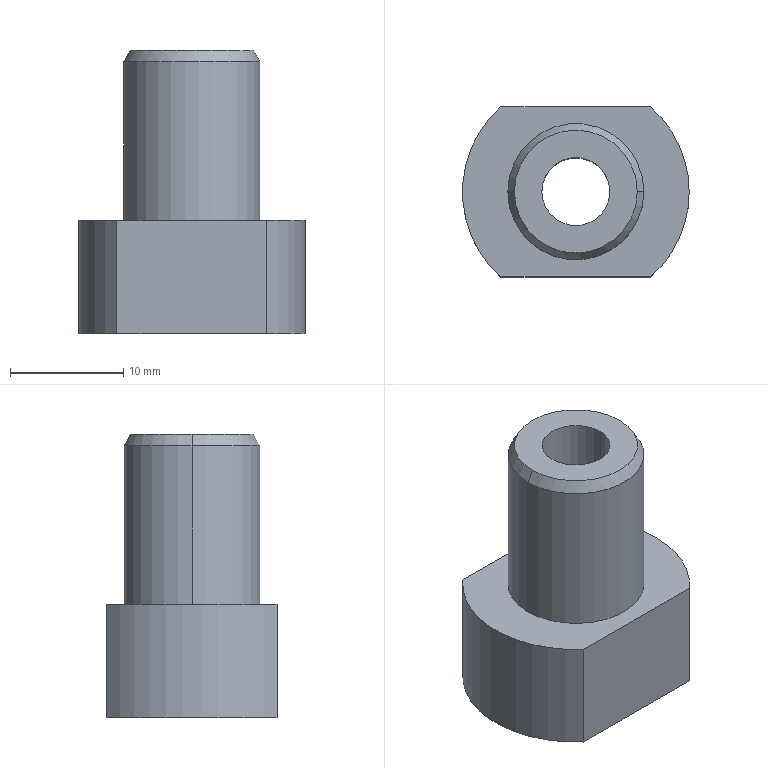Part | SolidWorks | features ICE 2, Chamfer 1, Extrusion 1 | 1 solid | 14 faces | box 20 x 15 x 25 mm | volume 3667 mm3 | cylinder 7 | plane 5 | cone 2 | commonest cylinder face diameters 20 x3 6 x2 12 x2
STEP:
#1=CARTESIAN_POINT('',(10.,0.,-10.));
#2=VERTEX_POINT('',#1);
#3=CARTESIAN_POINT('',(6.614,-7.5,-10.));
#4=VERTEX_POINT('',#3);
#5=CARTESIAN_POINT('',(0.,0.,-10.));
#6=DIRECTION('',(0.,0.,-1.));
#7=DIRECTION('',(-1.,0.,0.));
#8=AXIS2_PLACEMENT_3D('',#5,#6,#7);
#9=CIRCLE('',#8,10.);
#10=EDGE_CURVE('',#2,#4,#9,.T.);
#11=ORIENTED_EDGE('',*,*,#10,.F.);
#12=CARTESIAN_POINT('',(10.,0.,0.));
#13=VERTEX_POINT('',#12);
#14=CARTESIAN_POINT('',(10.,0.,-10.));
#15=DIRECTION('',(0.,0.,1.));
#16=VECTOR('',#15,1000.);
#17=LINE('',#14,#16);
#18=EDGE_CURVE('',#2,#13,#17,.T.);
#19=ORIENTED_EDGE('',*,*,#18,.T.);
#20=CARTESIAN_POINT('',(6.614,-7.5,0.));
#21=VERTEX_POINT('',#20);
#22=CARTESIAN_POINT('',(0.,0.,0.));
#23=DIRECTION('',(0.,0.,-1.));
#24=DIRECTION('',(-1.,0.,0.));
#25=AXIS2_PLACEMENT_3D('',#22,#23,#24);
#26=CIRCLE('',#25,10.);
#27=EDGE_CURVE('',#13,#21,#26,.T.);
#28=ORIENTED_EDGE('',*,*,#27,.T.);
#29=CARTESIAN_POINT('',(6.614,-7.5,-10.));
#30=DIRECTION('',(0.,0.,-1.));
#31=VECTOR('',#30,1000.);
#32=LINE('',#29,#31);
#33=EDGE_CURVE('',#21,#4,#32,.T.);
#34=ORIENTED_EDGE('',*,*,#33,.T.);
#35=EDGE_LOOP('',(#11,#19,#28,#34));
#36=FACE_OUTER_BOUND('',#35,.T.);
#37=CARTESIAN_POINT('',(0.,0.,-10.));
#38=DIRECTION('',(0.,0.,1.));
#39=DIRECTION('',(1.,0.,0.));
#40=AXIS2_PLACEMENT_3D('',#37,#38,#39);
#41=CYLINDRICAL_SURFACE('',#40,10.);
#42=ADVANCED_FACE('',(#36),#41,.T.);
#43=CARTESIAN_POINT('',(5.423,0.,15.));
#44=VERTEX_POINT('',#43);
#45=CARTESIAN_POINT('',(-5.423,0.,15.));
#46=VERTEX_POINT('',#45);
#47=CARTESIAN_POINT('',(0.,0.,15.));
#48=DIRECTION('',(0.,0.,1.));
#49=DIRECTION('',(1.,0.,0.));
#50=AXIS2_PLACEMENT_3D('',#47,#48,#49);
#51=CIRCLE('',#50,5.423);
#52=EDGE_CURVE('',#44,#46,#51,.T.);
#53=ORIENTED_EDGE('',*,*,#52,.F.);
#54=CARTESIAN_POINT('',(6.,0.,14.));
#55=VERTEX_POINT('',#54);
#56=CARTESIAN_POINT('',(5.423,0.,15.));
#57=DIRECTION('',(0.5,0.,-0.866));
#58=VECTOR('',#57,1000.);
#59=LINE('',#56,#58);
#60=EDGE_CURVE('',#44,#55,#59,.T.);
#61=ORIENTED_EDGE('',*,*,#60,.T.);
#62=CARTESIAN_POINT('',(-6.,0.,14.));
#63=VERTEX_POINT('',#62);
#64=CARTESIAN_POINT('',(0.,0.,14.));
#65=DIRECTION('',(0.,0.,-1.));
#66=DIRECTION('',(1.,0.,0.));
#67=AXIS2_PLACEMENT_3D('',#64,#65,#66);
#68=CIRCLE('',#67,6.);
#69=EDGE_CURVE('',#63,#55,#68,.T.);
#70=ORIENTED_EDGE('',*,*,#69,.F.);
#71=CARTESIAN_POINT('',(-5.423,0.,15.));
#72=DIRECTION('',(-0.5,0.,-0.866));
#73=VECTOR('',#72,1000.);
#74=LINE('',#71,#73);
#75=EDGE_CURVE('',#46,#63,#74,.T.);
#76=ORIENTED_EDGE('',*,*,#75,.F.);
#77=EDGE_LOOP('',(#53,#61,#70,#76));
#78=FACE_OUTER_BOUND('',#77,.T.);
#79=CARTESIAN_POINT('',(0.,0.,15.));
#80=DIRECTION('',(0.,0.,-1.));
#81=DIRECTION('',(-1.,0.,0.));
#82=AXIS2_PLACEMENT_3D('',#79,#80,#81);
#83=CONICAL_SURFACE('',#82,5.423,0.5236);
#84=ADVANCED_FACE('',(#78),#83,.T.);
#85=CARTESIAN_POINT('',(-3.,0.,15.));
#86=VERTEX_POINT('',#85);
#87=CARTESIAN_POINT('',(3.,0.,15.));
#88=VERTEX_POINT('',#87);
#89=CARTESIAN_POINT('',(0.,0.,15.));
#90=DIRECTION('',(0.,0.,1.));
#91=DIRECTION('',(1.,0.,0.));
#92=AXIS2_PLACEMENT_3D('',#89,#90,#91);
#93=CIRCLE('',#92,3.);
#94=EDGE_CURVE('',#86,#88,#93,.T.);
#95=ORIENTED_EDGE('',*,*,#94,.T.);
#96=CARTESIAN_POINT('',(3.,0.,-10.));
#97=VERTEX_POINT('',#96);
#98=CARTESIAN_POINT('',(3.,0.,15.));
#99=DIRECTION('',(0.,0.,-1.));
#100=VECTOR('',#99,1000.);
#101=LINE('',#98,#100);
#102=EDGE_CURVE('',#88,#97,#101,.T.);
#103=ORIENTED_EDGE('',*,*,#102,.T.);
#104=CARTESIAN_POINT('',(-3.,0.,-10.));
#105=VERTEX_POINT('',#104);
#106=CARTESIAN_POINT('',(0.,0.,-10.));
#107=DIRECTION('',(0.,0.,-1.));
#108=DIRECTION('',(-1.,0.,0.));
#109=AXIS2_PLACEMENT_3D('',#106,#107,#108);
#110=CIRCLE('',#109,3.);
#111=EDGE_CURVE('',#97,#105,#110,.T.);
#112=ORIENTED_EDGE('',*,*,#111,.T.);
#113=CARTESIAN_POINT('',(-3.,0.,15.));
#114=DIRECTION('',(0.,0.,-1.));
#115=VECTOR('',#114,1000.);
#116=LINE('',#113,#115);
#117=EDGE_CURVE('',#86,#105,#116,.T.);
#118=ORIENTED_EDGE('',*,*,#117,.F.);
#119=EDGE_LOOP('',(#95,#103,#112,#118));
#120=FACE_OUTER_BOUND('',#119,.T.);
#121=CARTESIAN_POINT('',(0.,0.,15.));
#122=DIRECTION('',(0.,0.,-1.));
#123=DIRECTION('',(-1.,0.,0.));
#124=AXIS2_PLACEMENT_3D('',#121,#122,#123);
#125=CYLINDRICAL_SURFACE('',#124,3.);
#126=ADVANCED_FACE('',(#120),#125,.F.);
#127=ORIENTED_EDGE('',*,*,#69,.T.);
#128=CARTESIAN_POINT('',(6.,0.,0.));
#129=VERTEX_POINT('',#128);
#130=CARTESIAN_POINT('',(6.,0.,15.));
#131=DIRECTION('',(0.,0.,-1.));
#132=VECTOR('',#131,1000.);
#133=LINE('',#130,#132);
#134=EDGE_CURVE('',#55,#129,#133,.T.);
#135=ORIENTED_EDGE('',*,*,#134,.T.);
#136=CARTESIAN_POINT('',(-6.,0.,0.));
#137=VERTEX_POINT('',#136);
#138=CARTESIAN_POINT('',(0.,0.,0.));
#139=DIRECTION('',(0.,0.,1.));
#140=DIRECTION('',(1.,0.,0.));
#141=AXIS2_PLACEMENT_3D('',#138,#139,#140);
#142=CIRCLE('',#141,6.);
#143=EDGE_CURVE('',#129,#137,#142,.T.);
#144=ORIENTED_EDGE('',*,*,#143,.T.);
#145=CARTESIAN_POINT('',(-6.,0.,15.));
#146=DIRECTION('',(0.,0.,-1.));
#147=VECTOR('',#146,1000.);
#148=LINE('',#145,#147);
#149=EDGE_CURVE('',#63,#137,#148,.T.);
#150=ORIENTED_EDGE('',*,*,#149,.F.);
#151=EDGE_LOOP('',(#127,#135,#144,#150));
#152=FACE_OUTER_BOUND('',#151,.T.);
#153=CARTESIAN_POINT('',(0.,0.,15.));
#154=DIRECTION('',(0.,0.,-1.));
#155=DIRECTION('',(-1.,0.,0.));
#156=AXIS2_PLACEMENT_3D('',#153,#154,#155);
#157=CYLINDRICAL_SURFACE('',#156,6.);
#158=ADVANCED_FACE('',(#152),#157,.T.);
#159=CARTESIAN_POINT('',(-6.614,-7.5,-10.));
#160=VERTEX_POINT('',#159);
#161=CARTESIAN_POINT('',(-6.614,7.5,-10.));
#162=VERTEX_POINT('',#161);
#163=CARTESIAN_POINT('',(0.,0.,-10.));
#164=DIRECTION('',(0.,0.,-1.));
#165=DIRECTION('',(-1.,0.,0.));
#166=AXIS2_PLACEMENT_3D('',#163,#164,#165);
#167=CIRCLE('',#166,10.);
#168=EDGE_CURVE('',#160,#162,#167,.T.);
#169=ORIENTED_EDGE('',*,*,#168,.F.);
#170=CARTESIAN_POINT('',(-6.614,-7.5,0.));
#171=VERTEX_POINT('',#170);
#172=CARTESIAN_POINT('',(-6.614,-7.5,-10.));
#173=DIRECTION('',(0.,0.,1.));
#174=VECTOR('',#173,1000.);
#175=LINE('',#172,#174);
#176=EDGE_CURVE('',#160,#171,#175,.T.);
#177=ORIENTED_EDGE('',*,*,#176,.T.);
#178=CARTESIAN_POINT('',(-6.614,7.5,0.));
#179=VERTEX_POINT('',#178);
#180=CARTESIAN_POINT('',(0.,0.,0.));
#181=DIRECTION('',(0.,0.,-1.));
#182=DIRECTION('',(-1.,0.,0.));
#183=AXIS2_PLACEMENT_3D('',#180,#181,#182);
#184=CIRCLE('',#183,10.);
#185=EDGE_CURVE('',#171,#179,#184,.T.);
#186=ORIENTED_EDGE('',*,*,#185,.T.);
#187=CARTESIAN_POINT('',(-6.614,7.5,-10.));
#188=DIRECTION('',(0.,0.,-1.));
#189=VECTOR('',#188,1000.);
#190=LINE('',#187,#189);
#191=EDGE_CURVE('',#179,#162,#190,.T.);
#192=ORIENTED_EDGE('',*,*,#191,.T.);
#193=EDGE_LOOP('',(#169,#177,#186,#192));
#194=FACE_OUTER_BOUND('',#193,.T.);
#195=CARTESIAN_POINT('',(0.,0.,-10.));
#196=DIRECTION('',(0.,0.,1.));
#197=DIRECTION('',(1.,0.,0.));
#198=AXIS2_PLACEMENT_3D('',#195,#196,#197);
#199=CYLINDRICAL_SURFACE('',#198,10.);
#200=ADVANCED_FACE('',(#194),#199,.T.);
#201=CARTESIAN_POINT('',(0.,0.,15.));
#202=DIRECTION('',(0.,0.,1.));
#203=DIRECTION('',(1.,0.,0.));
#204=AXIS2_PLACEMENT_3D('',#201,#202,#203);
#205=CIRCLE('',#204,5.423);
#206=EDGE_CURVE('',#46,#44,#205,.T.);
#207=ORIENTED_EDGE('',*,*,#206,.T.);
#208=ORIENTED_EDGE('',*,*,#52,.T.);
#209=EDGE_LOOP('',(#207,#208));
#210=FACE_OUTER_BOUND('',#209,.T.);
#211=ORIENTED_EDGE('',*,*,#94,.F.);
#212=CARTESIAN_POINT('',(0.,0.,15.));
#213=DIRECTION('',(0.,0.,1.));
#214=DIRECTION('',(1.,0.,0.));
#215=AXIS2_PLACEMENT_3D('',#212,#213,#214);
#216=CIRCLE('',#215,3.);
#217=EDGE_CURVE('',#88,#86,#216,.T.);
#218=ORIENTED_EDGE('',*,*,#217,.F.);
#219=EDGE_LOOP('',(#211,#218));
#220=FACE_BOUND('',#219,.T.);
#221=CARTESIAN_POINT('',(0.,0.,15.));
#222=DIRECTION('',(0.,0.,1.));
#223=DIRECTION('',(1.,0.,0.));
#224=AXIS2_PLACEMENT_3D('',#221,#222,#223);
#225=PLANE('',#224);
#226=ADVANCED_FACE('',(#210,#220),#225,.T.);
#227=ORIENTED_EDGE('',*,*,#134,.F.);
#228=CARTESIAN_POINT('',(0.,0.,14.));
#229=DIRECTION('',(0.,0.,-1.));
#230=DIRECTION('',(1.,0.,0.));
#231=AXIS2_PLACEMENT_3D('',#228,#229,#230);
#232=CIRCLE('',#231,6.);
#233=EDGE_CURVE('',#55,#63,#232,.T.);
#234=ORIENTED_EDGE('',*,*,#233,.T.);
#235=ORIENTED_EDGE('',*,*,#149,.T.);
#236=CARTESIAN_POINT('',(0.,0.,0.));
#237=DIRECTION('',(0.,0.,1.));
#238=DIRECTION('',(1.,0.,0.));
#239=AXIS2_PLACEMENT_3D('',#236,#237,#238);
#240=CIRCLE('',#239,6.);
#241=EDGE_CURVE('',#137,#129,#240,.T.);
#242=ORIENTED_EDGE('',*,*,#241,.T.);
#243=EDGE_LOOP('',(#227,#234,#235,#242));
#244=FACE_OUTER_BOUND('',#243,.T.);
#245=CARTESIAN_POINT('',(0.,0.,15.));
#246=DIRECTION('',(0.,0.,-1.));
#247=DIRECTION('',(-1.,0.,0.));
#248=AXIS2_PLACEMENT_3D('',#245,#246,#247);
#249=CYLINDRICAL_SURFACE('',#248,6.);
#250=ADVANCED_FACE('',(#244),#249,.T.);
#251=ORIENTED_EDGE('',*,*,#102,.F.);
#252=ORIENTED_EDGE('',*,*,#217,.T.);
#253=ORIENTED_EDGE('',*,*,#117,.T.);
#254=CARTESIAN_POINT('',(0.,0.,-10.));
#255=DIRECTION('',(0.,0.,-1.));
#256=DIRECTION('',(-1.,0.,0.));
#257=AXIS2_PLACEMENT_3D('',#254,#255,#256);
#258=CIRCLE('',#257,3.);
#259=EDGE_CURVE('',#105,#97,#258,.T.);
#260=ORIENTED_EDGE('',*,*,#259,.T.);
#261=EDGE_LOOP('',(#251,#252,#253,#260));
#262=FACE_OUTER_BOUND('',#261,.T.);
#263=CARTESIAN_POINT('',(0.,0.,15.));
#264=DIRECTION('',(0.,0.,-1.));
#265=DIRECTION('',(-1.,0.,0.));
#266=AXIS2_PLACEMENT_3D('',#263,#264,#265);
#267=CYLINDRICAL_SURFACE('',#266,3.);
#268=ADVANCED_FACE('',(#262),#267,.F.);
#269=ORIENTED_EDGE('',*,*,#60,.F.);
#270=ORIENTED_EDGE('',*,*,#206,.F.);
#271=ORIENTED_EDGE('',*,*,#75,.T.);
#272=ORIENTED_EDGE('',*,*,#233,.F.);
#273=EDGE_LOOP('',(#269,#270,#271,#272));
#274=FACE_OUTER_BOUND('',#273,.T.);
#275=CARTESIAN_POINT('',(0.,0.,15.));
#276=DIRECTION('',(0.,0.,-1.));
#277=DIRECTION('',(-1.,0.,0.));
#278=AXIS2_PLACEMENT_3D('',#275,#276,#277);
#279=CONICAL_SURFACE('',#278,5.423,0.5236);
#280=ADVANCED_FACE('',(#274),#279,.T.);
#281=CARTESIAN_POINT('',(12.433,-7.5,-10.));
#282=DIRECTION('',(1.,0.,0.));
#283=VECTOR('',#282,1000.);
#284=LINE('',#281,#283);
#285=EDGE_CURVE('',#160,#4,#284,.T.);
#286=ORIENTED_EDGE('',*,*,#285,.F.);
#287=ORIENTED_EDGE('',*,*,#168,.T.);
#288=CARTESIAN_POINT('',(6.614,7.5,-10.));
#289=VERTEX_POINT('',#288);
#290=CARTESIAN_POINT('',(12.433,7.5,-10.));
#291=DIRECTION('',(-1.,0.,0.));
#292=VECTOR('',#291,1000.);
#293=LINE('',#290,#292);
#294=EDGE_CURVE('',#289,#162,#293,.T.);
#295=ORIENTED_EDGE('',*,*,#294,.F.);
#296=CARTESIAN_POINT('',(0.,0.,-10.));
#297=DIRECTION('',(0.,0.,-1.));
#298=DIRECTION('',(-1.,0.,0.));
#299=AXIS2_PLACEMENT_3D('',#296,#297,#298);
#300=CIRCLE('',#299,10.);
#301=EDGE_CURVE('',#289,#2,#300,.T.);
#302=ORIENTED_EDGE('',*,*,#301,.T.);
#303=ORIENTED_EDGE('',*,*,#10,.T.);
#304=EDGE_LOOP('',(#286,#287,#295,#302,#303));
#305=FACE_OUTER_BOUND('',#304,.T.);
#306=ORIENTED_EDGE('',*,*,#259,.F.);
#307=ORIENTED_EDGE('',*,*,#111,.F.);
#308=EDGE_LOOP('',(#306,#307));
#309=FACE_BOUND('',#308,.T.);
#310=CARTESIAN_POINT('',(0.,0.,-10.));
#311=DIRECTION('',(0.,0.,-1.));
#312=DIRECTION('',(-1.,0.,0.));
#313=AXIS2_PLACEMENT_3D('',#310,#311,#312);
#314=PLANE('',#313);
#315=ADVANCED_FACE('',(#305,#309),#314,.T.);
#316=ORIENTED_EDGE('',*,*,#241,.F.);
#317=ORIENTED_EDGE('',*,*,#143,.F.);
#318=EDGE_LOOP('',(#316,#317));
#319=FACE_BOUND('',#318,.T.);
#320=ORIENTED_EDGE('',*,*,#185,.F.);
#321=CARTESIAN_POINT('',(0.,-7.5,0.));
#322=DIRECTION('',(1.,0.,0.));
#323=VECTOR('',#322,1000.);
#324=LINE('',#321,#323);
#325=EDGE_CURVE('',#171,#21,#324,.T.);
#326=ORIENTED_EDGE('',*,*,#325,.T.);
#327=ORIENTED_EDGE('',*,*,#27,.F.);
#328=CARTESIAN_POINT('',(6.614,7.5,0.));
#329=VERTEX_POINT('',#328);
#330=CARTESIAN_POINT('',(0.,0.,0.));
#331=DIRECTION('',(0.,0.,-1.));
#332=DIRECTION('',(-1.,0.,0.));
#333=AXIS2_PLACEMENT_3D('',#330,#331,#332);
#334=CIRCLE('',#333,10.);
#335=EDGE_CURVE('',#329,#13,#334,.T.);
#336=ORIENTED_EDGE('',*,*,#335,.F.);
#337=CARTESIAN_POINT('',(0.,7.5,0.));
#338=DIRECTION('',(-1.,0.,0.));
#339=VECTOR('',#338,1000.);
#340=LINE('',#337,#339);
#341=EDGE_CURVE('',#329,#179,#340,.T.);
#342=ORIENTED_EDGE('',*,*,#341,.T.);
#343=EDGE_LOOP('',(#320,#326,#327,#336,#342));
#344=FACE_OUTER_BOUND('',#343,.T.);
#345=CARTESIAN_POINT('',(0.,0.,0.));
#346=DIRECTION('',(0.,0.,-1.));
#347=DIRECTION('',(-1.,0.,0.));
#348=AXIS2_PLACEMENT_3D('',#345,#346,#347);
#349=PLANE('',#348);
#350=ADVANCED_FACE('',(#319,#344),#349,.F.);
#351=ORIENTED_EDGE('',*,*,#18,.F.);
#352=ORIENTED_EDGE('',*,*,#301,.F.);
#353=CARTESIAN_POINT('',(6.614,7.5,-10.));
#354=DIRECTION('',(0.,0.,1.));
#355=VECTOR('',#354,1000.);
#356=LINE('',#353,#355);
#357=EDGE_CURVE('',#289,#329,#356,.T.);
#358=ORIENTED_EDGE('',*,*,#357,.T.);
#359=ORIENTED_EDGE('',*,*,#335,.T.);
#360=EDGE_LOOP('',(#351,#352,#358,#359));
#361=FACE_OUTER_BOUND('',#360,.T.);
#362=CARTESIAN_POINT('',(0.,0.,-10.));
#363=DIRECTION('',(0.,0.,1.));
#364=DIRECTION('',(1.,0.,0.));
#365=AXIS2_PLACEMENT_3D('',#362,#363,#364);
#366=CYLINDRICAL_SURFACE('',#365,10.);
#367=ADVANCED_FACE('',(#361),#366,.T.);
#368=ORIENTED_EDGE('',*,*,#294,.T.);
#369=ORIENTED_EDGE('',*,*,#191,.F.);
#370=ORIENTED_EDGE('',*,*,#341,.F.);
#371=ORIENTED_EDGE('',*,*,#357,.F.);
#372=EDGE_LOOP('',(#368,#369,#370,#371));
#373=FACE_OUTER_BOUND('',#372,.T.);
#374=CARTESIAN_POINT('',(12.433,7.5,15.));
#375=DIRECTION('',(0.,-1.,0.));
#376=DIRECTION('',(0.,0.,-1.));
#377=AXIS2_PLACEMENT_3D('',#374,#375,#376);
#378=PLANE('',#377);
#379=ADVANCED_FACE('',(#373),#378,.F.);
#380=ORIENTED_EDGE('',*,*,#285,.T.);
#381=ORIENTED_EDGE('',*,*,#33,.F.);
#382=ORIENTED_EDGE('',*,*,#325,.F.);
#383=ORIENTED_EDGE('',*,*,#176,.F.);
#384=EDGE_LOOP('',(#380,#381,#382,#383));
#385=FACE_OUTER_BOUND('',#384,.T.);
#386=CARTESIAN_POINT('',(12.433,-7.5,15.));
#387=DIRECTION('',(0.,1.,0.));
#388=DIRECTION('',(0.,0.,1.));
#389=AXIS2_PLACEMENT_3D('',#386,#387,#388);
#390=PLANE('',#389);
#391=ADVANCED_FACE('',(#385),#390,.F.);
#392=CLOSED_SHELL('',(#42,#84,#126,#158,#200,#226,#250,#268,#280,#315,#350,#367,#379,#391));
#393=MANIFOLD_SOLID_BREP('',#392);
#394=CARTESIAN_POINT('',(0.,0.,0.));
#395=DIRECTION('',(0.,0.,1.));
#396=DIRECTION('',(1.,0.,0.));
#397=AXIS2_PLACEMENT_3D('',#394,#395,#396);
#398=(LENGTH_UNIT()NAMED_UNIT(*)SI_UNIT(.MILLI.,.METRE.));
#399=UNCERTAINTY_MEASURE_WITH_UNIT(LENGTH_MEASURE(0.00001),#398,'','');
#400=(NAMED_UNIT(*)PLANE_ANGLE_UNIT()SI_UNIT($,.RADIAN.));
#401=(NAMED_UNIT(*)SI_UNIT($,.STERADIAN.)SOLID_ANGLE_UNIT());
#402=(GEOMETRIC_REPRESENTATION_CONTEXT(3)GLOBAL_UNCERTAINTY_ASSIGNED_CONTEXT((#399))GLOBAL_UNIT_ASSIGNED_CONTEXT((#398,#400,#401))REPRESENTATION_CONTEXT('',''));
#403=ADVANCED_BREP_SHAPE_REPRESENTATION('',(#393,#397),#402);